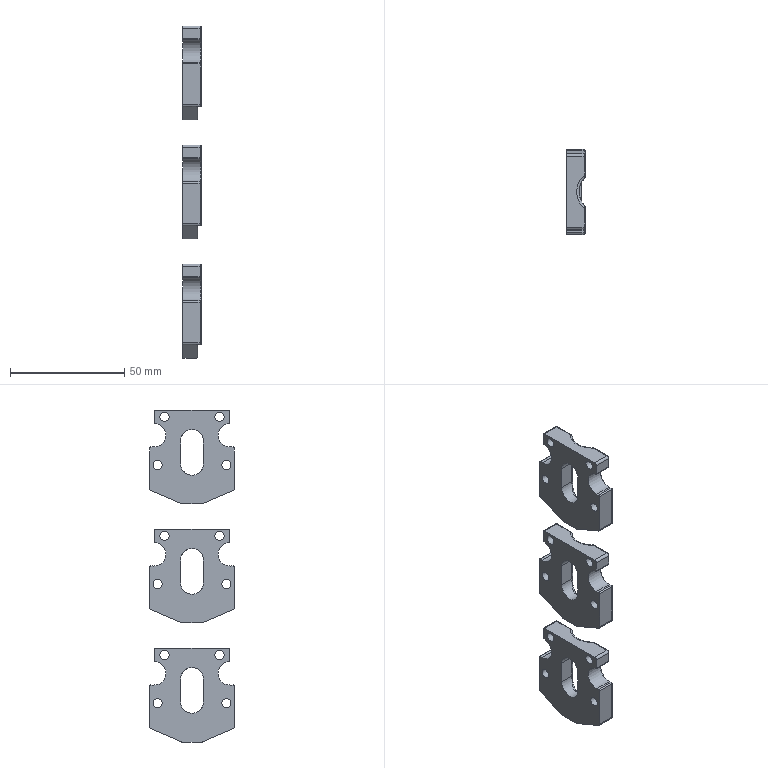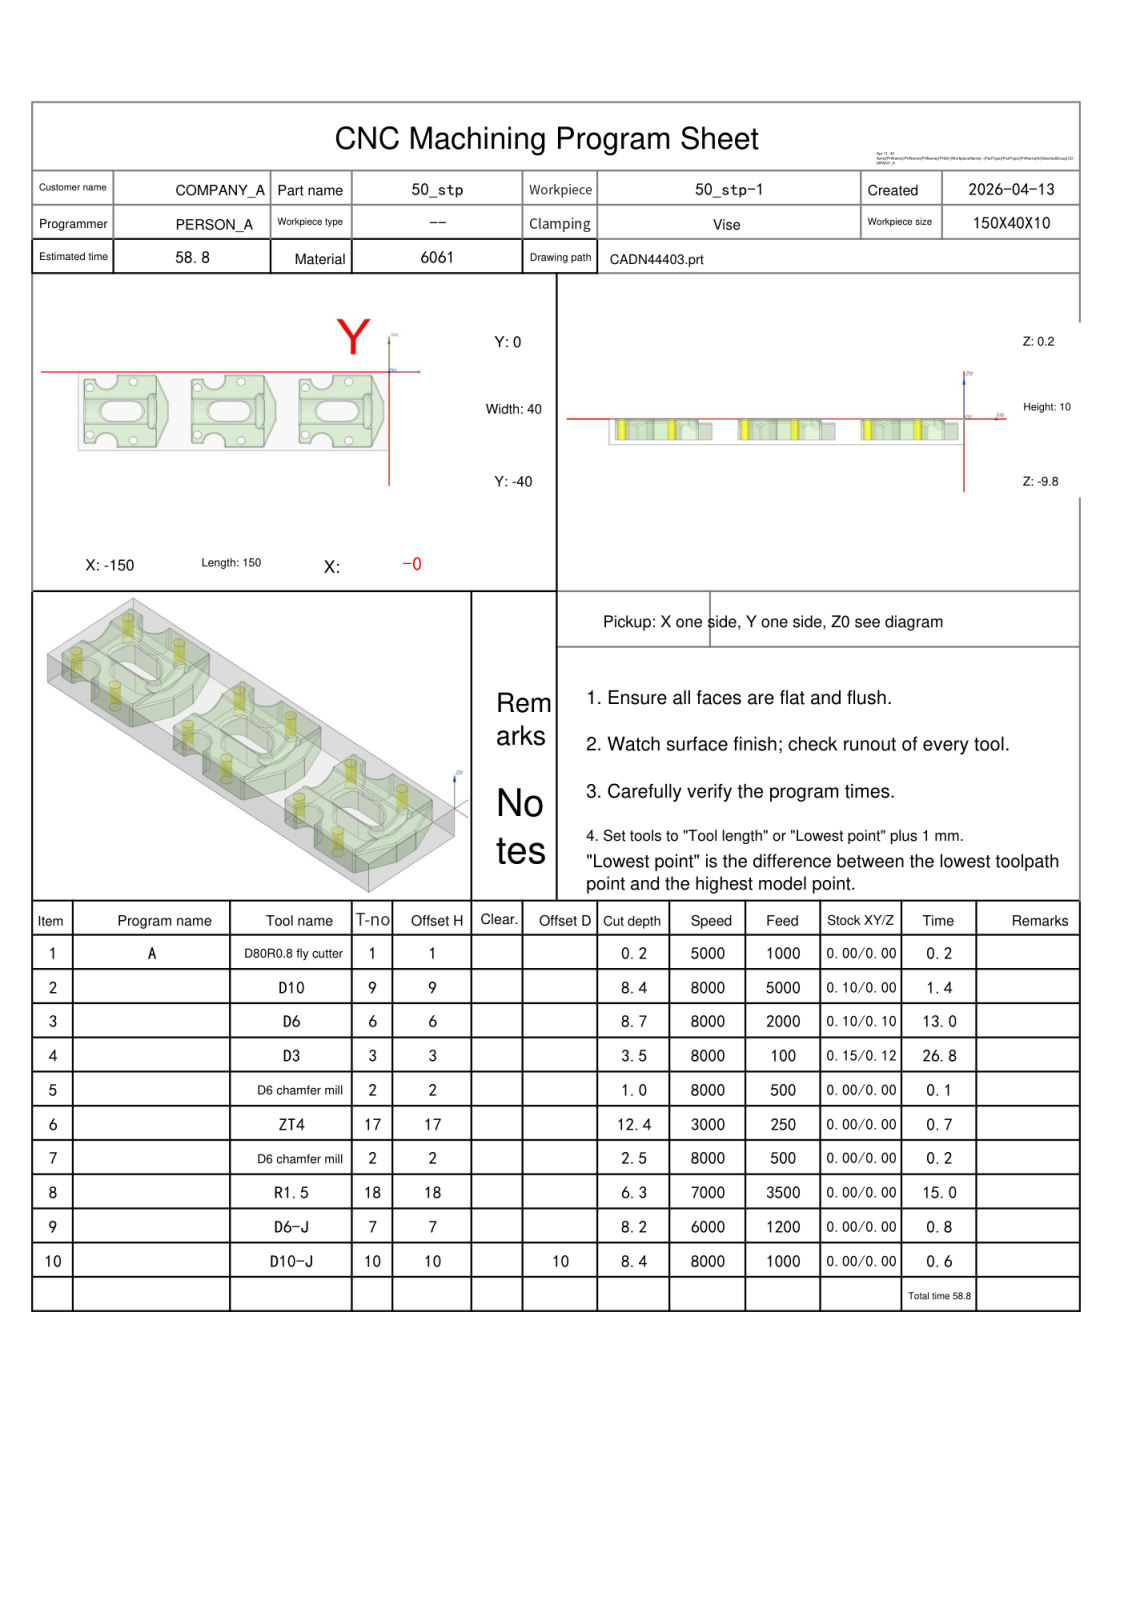NC program | NX | posted by the shop | part box 8 x 37 x 145 mm
Lines 1 to 1271 of 223411:
%
O0001
(Machine time: 60.56 MIN)
(===Total Tool:9===)
(T1=D80R0.8 fly cutter D=80.  R=0.8  D-  H01 Z=-0.   )
(T9=D10     D=10.  R=0.   D-  H09 Z=-8.2  )
(T6=D6      D=6.   R=0.   D-  H06 Z=-8.5  )
(T3=D3      D=3.   R=0.   D-  H03 Z=-3.31 )
(T2=D6 chamfer mill   D=6.   R=0.   D-  H02 Z=-2.3  )
(T17=ZT4    D=4.   DR_a=118 D-  H17 Z=-12.2 )
(T18=R1.5   D=3.   R=1.5  D-  H18 Z=-6.09 )
(T7=D6-J    D=6.   R=0.   D7  H07 Z=-8.   )
(T10=D10-J  D=10.  R=0.   D10 H10 Z=-8.2  )
G80 G90 G17 G49 G40
G91 G28 Z0
M01
N1 T01 M06
(D80R0.8 fly cutter  D=80. R=0.8 H=01 ce=0.00 di=0.00)
G00 G90 G54 X-192.5 Y-20. M03 S5000
G43 H01 Z20.
M08
Z2.
G01 Z0.0 F1000.
X-187.5
X37.5
X42.5
Z2.
G00 Z20.
G91 G28 Z0.0
M05
M09
G91 G28 Z0.0
M01
N2 T09 M06
(D10  D=10. R=0. H=09 ce=0.10 di=0.00)
G00 G90 G54 X-48.6 Y-20. M03 S8000
G43 H09 Z20.
M08
Z0.0
G01 Y-4.5 Z-.061 F5000.
G02 X-42.5 Y1.6 Z-.099 I6.1 J0.0
G01 X-38.128 Z-.117
G02 X-32.55 Y-3.504 Z-.149 I0.0 J-5.6
G01 X-32.549 Y-3.534
X-32.525 Y-3.554 Z-.15
X-32.496 Y-3.55
X-32.466
X-32.446 Y-3.527
X-32.45 Y-3.497
X-32.514 Y-2.3 Z-.155
G02 X-27.223 Y3.592 Z-.19 I5.592 J.3
X-26.922 Y3.6 Z-.191 I.3 J-5.592
G01 X-9.159 Z-.261
G02 X-3.553 Y-.097 Z-.289 I0.0 J-6.1
G01 X2.147 Y-13.397 Z-.346
G02 X2.6 Y-15.603 Z-.355 I-5.147 J-2.206
G01 Y-24.397 Z-.39
G02 X2.147 Y-26.603 Z-.399 I-5.6 J0.0
G01 X-3.553 Y-39.903 Z-.456
G02 X-9.159 Y-43.6 Z-.484 I-5.607 J2.403
G01 X-26.922 Z-.555
G02 X-32.522 Y-38. Z-.59 I0.0 J5.6
X-32.514 Y-37.7 Z-.591 I5.6 J0.0
G01 X-32.45 Y-36.503 Z-.595
X-32.447 Y-36.473 Z-.596
X-32.467 Y-36.45
X-32.497
X-32.527 Y-36.446
X-32.55 Y-36.466
Y-36.496
G02 X-38.128 Y-41.6 Z-.629 I-5.578 J.496
G01 X-42.5 Z-.646
G02 X-48.6 Y-35.5 Z-.684 I0.0 J6.1
G01 Y-4.5 Z-.807
G02 X-42.5 Y1.6 Z-.845 I6.1 J0.0
G01 X-38.128 Z-.862
G02 X-32.55 Y-3.504 Z-.895 I0.0 J-5.6
G01 X-32.549 Y-3.534
X-32.525 Y-3.554
X-32.496 Y-3.55
X-32.466
X-32.446 Y-3.527
X-32.45 Y-3.497
X-32.514 Y-2.3 Z-.9
G02 X-27.223 Y3.592 Z-.935 I5.592 J.3
X-26.922 Y3.6 Z-.936 I.3 J-5.592
G01 X-9.159 Z-1.006
G02 X-3.553 Y-.097 Z-1.035 I0.0 J-6.1
G01 X2.147 Y-13.397 Z-1.092
G02 X2.6 Y-15.603 Z-1.101 I-5.147 J-2.206
G01 Y-24.397 Z-1.136
G02 X2.147 Y-26.603 Z-1.145 I-5.6 J0.0
G01 X-3.553 Y-39.903 Z-1.202
G02 X-9.159 Y-43.6 Z-1.23 I-5.607 J2.403
G01 X-26.922 Z-1.3
G02 X-32.522 Y-38. Z-1.335 I0.0 J5.6
X-32.514 Y-37.7 Z-1.336 I5.6 J0.0
G01 X-32.45 Y-36.503 Z-1.341
X-32.447 Y-36.473
X-32.467 Y-36.45
X-32.497
X-32.527 Y-36.446
X-32.55 Y-36.466
Y-36.496 Z-1.342
G02 X-38.128 Y-41.6 Z-1.374 I-5.578 J.496
G01 X-42.5 Z-1.392
G02 X-48.6 Y-35.5 Z-1.43 I0.0 J6.1
G01 Y-4.5 Z-1.552
G02 X-42.5 Y1.6 Z-1.59 I6.1 J0.0
G01 X-38.128 Z-1.607
G02 X-32.55 Y-3.504 Z-1.64 I0.0 J-5.6
G01 X-32.549 Y-3.534
X-32.525 Y-3.554
X-32.496 Y-3.55 Z-1.641
X-32.466
X-32.446 Y-3.527
X-32.45 Y-3.497
X-32.514 Y-2.3 Z-1.646
G02 X-27.223 Y3.592 Z-1.68 I5.592 J.3
X-26.922 Y3.6 Z-1.682 I.3 J-5.592
G01 X-9.159 Z-1.752
G02 X-3.553 Y-.097 Z-1.78 I0.0 J-6.1
G01 X2.147 Y-13.397 Z-1.837
G02 X2.6 Y-15.603 Z-1.846 I-5.147 J-2.206
G01 Y-24.397 Z-1.881
G02 X2.147 Y-26.603 Z-1.89 I-5.6 J0.0
G01 X-3.553 Y-39.903 Z-1.947
G02 X-9.159 Y-43.6 Z-1.975 I-5.607 J2.403
G01 X-26.922 Z-2.046
G02 X-32.522 Y-38. Z-2.08 I0.0 J5.6
X-32.514 Y-37.7 Z-2.082 I5.6 J0.0
G01 X-32.45 Y-36.503 Z-2.086
X-32.447 Y-36.473
X-32.467 Y-36.45 Z-2.087
X-32.497
X-32.527 Y-36.446
X-32.55 Y-36.466
Y-36.496
G02 X-38.128 Y-41.6 Z-2.12 I-5.578 J.496
G01 X-42.5 Z-2.137
G02 X-48.6 Y-35.5 Z-2.175 I0.0 J6.1
G01 Y-4.5 Z-2.298
G02 X-42.5 Y1.6 Z-2.336 I6.1 J0.0
G01 X-38.128 Z-2.353
G02 X-32.55 Y-3.504 Z-2.386 I0.0 J-5.6
G01 X-32.549 Y-3.534
X-32.525 Y-3.554
X-32.496 Y-3.55
X-32.466
X-32.446 Y-3.527
X-32.45 Y-3.497
X-32.514 Y-2.3 Z-2.391
G02 X-27.223 Y3.592 Z-2.426 I5.592 J.3
X-26.922 Y3.6 Z-2.427 I.3 J-5.592
G01 X-9.159 Z-2.497
G02 X-3.553 Y-.097 Z-2.525 I0.0 J-6.1
G01 X2.147 Y-13.397 Z-2.583
G02 X2.6 Y-15.603 Z-2.592 I-5.147 J-2.206
G01 Y-24.397 Z-2.626
G02 X2.147 Y-26.603 Z-2.635 I-5.6 J0.0
G01 X-3.553 Y-39.903 Z-2.693
G02 X-9.159 Y-43.6 Z-2.721 I-5.607 J2.403
G01 X-26.922 Z-2.791
G02 X-32.522 Y-38. Z-2.826 I0.0 J5.6
X-32.514 Y-37.7 Z-2.827 I5.6 J0.0
G01 X-32.45 Y-36.503 Z-2.832
X-32.447 Y-36.473
X-32.467 Y-36.45
X-32.497
X-32.527 Y-36.446
X-32.55 Y-36.466
Y-36.496
G02 X-38.128 Y-41.6 Z-2.865 I-5.578 J.496
G01 X-42.5 Z-2.883
G02 X-48.6 Y-35.5 Z-2.92 I0.0 J6.1
G01 Y-4.5 Z-3.043
G02 X-42.5 Y1.6 Z-3.081 I6.1 J0.0
G01 X-38.128 Z-3.098
G02 X-32.55 Y-3.504 Z-3.131 I0.0 J-5.6
G01 X-32.549 Y-3.534
X-32.525 Y-3.554
X-32.496 Y-3.55
X-32.466 Z-3.132
X-32.446 Y-3.527
X-32.45 Y-3.497
X-32.514 Y-2.3 Z-3.137
G02 X-27.223 Y3.592 Z-3.171 I5.592 J.3
X-26.922 Y3.6 Z-3.173 I.3 J-5.592
G01 X-9.159 Z-3.243
G02 X-3.553 Y-.097 Z-3.271 I0.0 J-6.1
G01 X2.147 Y-13.397 Z-3.328
G02 X2.6 Y-15.603 Z-3.337 I-5.147 J-2.206
G01 Y-24.397 Z-3.372
G02 X2.147 Y-26.603 Z-3.381 I-5.6 J0.0
G01 X-3.553 Y-39.903 Z-3.438
G02 X-9.159 Y-43.6 Z-3.466 I-5.607 J2.403
G01 X-26.922 Z-3.537
G02 X-32.522 Y-38. Z-3.571 I0.0 J5.6
X-32.514 Y-37.7 Z-3.573 I5.6 J0.0
G01 X-32.45 Y-36.503 Z-3.577
X-32.447 Y-36.473
X-32.467 Y-36.45 Z-3.578
X-32.497
X-32.527 Y-36.446
X-32.55 Y-36.466
Y-36.496
G02 X-38.128 Y-41.6 Z-3.611 I-5.578 J.496
G01 X-42.5 Z-3.628
G02 X-48.6 Y-35.5 Z-3.666 I0.0 J6.1
G01 Y-4.5 Z-3.789
G02 X-42.5 Y1.6 Z-3.827 I6.1 J0.0
G01 X-38.128 Z-3.844
G02 X-32.55 Y-3.504 Z-3.877 I0.0 J-5.6
G01 X-32.549 Y-3.534
X-32.525 Y-3.554
X-32.496 Y-3.55
X-32.466
X-32.446 Y-3.527
X-32.45 Y-3.497
X-32.514 Y-2.3 Z-3.882
G02 X-27.223 Y3.592 Z-3.917 I5.592 J.3
X-26.922 Y3.6 Z-3.918 I.3 J-5.592
G01 X-9.159 Z-3.988
G02 X-3.553 Y-.097 Z-4.016 I0.0 J-6.1
G01 X2.147 Y-13.397 Z-4.074
G02 X2.6 Y-15.603 Z-4.083 I-5.147 J-2.206
G01 Y-24.397 Z-4.117
G02 X2.147 Y-26.603 Z-4.126 I-5.6 J0.0
G01 X-3.553 Y-39.903 Z-4.184
G02 X-9.159 Y-43.6 Z-4.212 I-5.607 J2.403
G01 X-26.922 Z-4.282
G02 X-32.522 Y-38. Z-4.317 I0.0 J5.6
X-32.514 Y-37.7 Z-4.318 I5.6 J0.0
G01 X-32.45 Y-36.503 Z-4.323
X-32.447 Y-36.473
X-32.467 Y-36.45
X-32.497
X-32.527 Y-36.446
X-32.55 Y-36.466
Y-36.496
G02 X-38.128 Y-41.6 Z-4.356 I-5.578 J.496
G01 X-42.5 Z-4.374
G02 X-48.6 Y-35.5 Z-4.411 I0.0 J6.1
G01 Y-4.5 Z-4.534
G02 X-42.5 Y1.6 Z-4.572 I6.1 J0.0
G01 X-38.128 Z-4.589
G02 X-32.55 Y-3.504 Z-4.622 I0.0 J-5.6
G01 X-32.549 Y-3.534
X-32.525 Y-3.554
X-32.496 Y-3.55
X-32.466 Z-4.623
X-32.446 Y-3.527
X-32.45 Y-3.497
X-32.514 Y-2.3 Z-4.627
G02 X-27.223 Y3.592 Z-4.662 I5.592 J.3
X-26.922 Y3.6 Z-4.663 I.3 J-5.592
G01 X-9.159 Z-4.734
G02 X-3.553 Y-.097 Z-4.762 I0.0 J-6.1
G01 X2.147 Y-13.397 Z-4.819
G02 X2.6 Y-15.603 Z-4.828 I-5.147 J-2.206
G01 Y-24.397 Z-4.863
G02 X2.147 Y-26.603 Z-4.872 I-5.6 J0.0
G01 X-3.553 Y-39.903 Z-4.929
G02 X-9.159 Y-43.6 Z-4.957 I-5.607 J2.403
G01 X-26.922 Z-5.027
G02 X-32.522 Y-38. Z-5.062 I0.0 J5.6
X-32.514 Y-37.7 Z-5.063 I5.6 J0.0
G01 X-32.45 Y-36.503 Z-5.068
X-32.447 Y-36.473
X-32.467 Y-36.45
X-32.497 Z-5.069
X-32.527 Y-36.446
X-32.55 Y-36.466
Y-36.496
G02 X-38.128 Y-41.6 Z-5.102 I-5.578 J.496
G01 X-42.5 Z-5.119
G02 X-48.6 Y-35.5 Z-5.157 I0.0 J6.1
G01 Y-4.5 Z-5.28
G02 X-42.5 Y1.6 Z-5.317 I6.1 J0.0
G01 X-38.128 Z-5.335
G02 X-32.55 Y-3.504 Z-5.368 I0.0 J-5.6
G01 X-32.549 Y-3.534
X-32.525 Y-3.554
X-32.496 Y-3.55
X-32.466
X-32.446 Y-3.527
X-32.45 Y-3.497
X-32.514 Y-2.3 Z-5.373
G02 X-27.223 Y3.592 Z-5.408 I5.592 J.3
X-26.922 Y3.6 Z-5.409 I.3 J-5.592
G01 X-9.159 Z-5.479
G02 X-3.553 Y-.097 Z-5.507 I0.0 J-6.1
G01 X2.147 Y-13.397 Z-5.565
G02 X2.6 Y-15.603 Z-5.574 I-5.147 J-2.206
G01 Y-24.397 Z-5.608
G02 X2.147 Y-26.603 Z-5.617 I-5.6 J0.0
G01 X-3.553 Y-39.903 Z-5.675
G02 X-9.159 Y-43.6 Z-5.703 I-5.607 J2.403
G01 X-26.922 Z-5.773
G02 X-32.522 Y-38. Z-5.808 I0.0 J5.6
X-32.514 Y-37.7 Z-5.809 I5.6 J0.0
G01 X-32.45 Y-36.503 Z-5.814
X-32.447 Y-36.473
X-32.467 Y-36.45
X-32.497
X-32.527 Y-36.446
X-32.55 Y-36.466
Y-36.496
G02 X-38.128 Y-41.6 Z-5.847 I-5.578 J.496
G01 X-42.5 Z-5.864
G02 X-48.6 Y-35.5 Z-5.902 I0.0 J6.1
G01 Y-4.5 Z-6.025
G02 X-42.5 Y1.6 Z-6.063 I6.1 J0.0
G01 X-38.128 Z-6.08
G02 X-32.55 Y-3.504 Z-6.113 I0.0 J-5.6
G01 X-32.549 Y-3.534
X-32.525 Y-3.554
X-32.496 Y-3.55
X-32.466
X-32.446 Y-3.527 Z-6.114
X-32.45 Y-3.497
X-32.514 Y-2.3 Z-6.118
G02 X-27.223 Y3.592 Z-6.153 I5.592 J.3
X-26.922 Y3.6 Z-6.154 I.3 J-5.592
G01 X-9.159 Z-6.225
G02 X-3.553 Y-.097 Z-6.253 I0.0 J-6.1
G01 X2.147 Y-13.397 Z-6.31
G02 X2.6 Y-15.603 Z-6.319 I-5.147 J-2.206
G01 Y-24.397 Z-6.354
G02 X2.147 Y-26.603 Z-6.363 I-5.6 J0.0
G01 X-3.553 Y-39.903 Z-6.42
G02 X-9.159 Y-43.6 Z-6.448 I-5.607 J2.403
G01 X-26.922 Z-6.518
G02 X-32.522 Y-38. Z-6.553 I0.0 J5.6
X-32.514 Y-37.7 Z-6.554 I5.6 J0.0
G01 X-32.45 Y-36.503 Z-6.559
X-32.447 Y-36.473
X-32.467 Y-36.45
X-32.497
X-32.527 Y-36.446 Z-6.56
X-32.55 Y-36.466
Y-36.496
G02 X-38.128 Y-41.6 Z-6.593 I-5.578 J.496
G01 X-42.5 Z-6.61
G02 X-48.6 Y-35.5 Z-6.648 I0.0 J6.1
G01 Y-4.5 Z-6.77
G02 X-42.5 Y1.6 Z-6.808 I6.1 J0.0
G01 X-38.128 Z-6.826
G02 X-32.55 Y-3.504 Z-6.858 I0.0 J-5.6
G01 X-32.549 Y-3.534 Z-6.859
X-32.525 Y-3.554
X-32.496 Y-3.55
X-32.466
X-32.446 Y-3.527
X-32.45 Y-3.497
X-32.514 Y-2.3 Z-6.864
G02 X-27.223 Y3.592 Z-6.899 I5.592 J.3
X-26.922 Y3.6 Z-6.9 I.3 J-5.592
G01 X-9.159 Z-6.97
G02 X-3.553 Y-.097 Z-6.998 I0.0 J-6.1
G01 X2.147 Y-13.397 Z-7.055
G02 X2.6 Y-15.603 Z-7.064 I-5.147 J-2.206
G01 Y-24.397 Z-7.099
G02 X2.147 Y-26.603 Z-7.108 I-5.6 J0.0
G01 X-3.553 Y-39.903 Z-7.165
G02 X-9.159 Y-43.6 Z-7.194 I-5.607 J2.403
G01 X-26.922 Z-7.264
G02 X-32.522 Y-38. Z-7.299 I0.0 J5.6
X-32.514 Y-37.7 Z-7.3 I5.6 J0.0
G01 X-32.45 Y-36.503 Z-7.305
X-32.447 Y-36.473
X-32.467 Y-36.45
X-32.497
X-32.527 Y-36.446
X-32.55 Y-36.466
Y-36.496
G02 X-38.128 Y-41.6 Z-7.338 I-5.578 J.496
G01 X-42.5 Z-7.355
G02 X-48.6 Y-35.5 Z-7.393 I0.0 J6.1
G01 Y-4.5 Z-7.516
G02 X-42.5 Y1.6 Z-7.554 I6.1 J0.0
G01 X-38.128 Z-7.571
G02 X-32.55 Y-3.504 Z-7.604 I0.0 J-5.6
G01 X-32.549 Y-3.534
X-32.525 Y-3.554
X-32.496 Y-3.55
X-32.466
X-32.446 Y-3.527
X-32.45 Y-3.497 Z-7.605
X-32.514 Y-2.3 Z-7.609
G02 X-27.223 Y3.592 Z-7.644 I5.592 J.3
X-26.922 Y3.6 Z-7.645 I.3 J-5.592
G01 X-9.159 Z-7.716
G02 X-3.553 Y-.097 Z-7.744 I0.0 J-6.1
G01 X2.147 Y-13.397 Z-7.801
G02 X2.6 Y-15.603 Z-7.81 I-5.147 J-2.206
G01 Y-24.397 Z-7.845
G02 X2.147 Y-26.603 Z-7.854 I-5.6 J0.0
G01 X-3.553 Y-39.903 Z-7.911
G02 X-9.159 Y-43.6 Z-7.939 I-5.607 J2.403
G01 X-26.922 Z-8.009
G02 X-32.522 Y-38. Z-8.044 I0.0 J5.6
X-32.514 Y-37.7 Z-8.045 I5.6 J0.0
G01 X-32.45 Y-36.503 Z-8.05
X-32.447 Y-36.473
X-32.467 Y-36.45
X-32.497
X-32.527 Y-36.446
X-32.55 Y-36.466 Z-8.051
Y-36.496
G02 X-38.128 Y-41.6 Z-8.083 I-5.578 J.496
G01 X-42.5 Z-8.101
G02 X-48.6 Y-35.5 Z-8.139 I0.0 J6.1
G01 Y-20. Z-8.2
Y-4.5
G02 X-42.5 Y1.6 I6.1 J0.0
G01 X-38.128
G02 X-32.55 Y-3.504 I0.0 J-5.6
G01 X-32.526 Y-3.554
X-32.467 Y-3.55
X-32.45 Y-3.497
X-32.514 Y-2.3
G02 X-32.522 Y-2. I5.592 J.3
X-26.922 Y3.6 I5.6 J0.0
G01 X-9.159
G02 X-3.553 Y-.097 I0.0 J-6.1
G01 X2.147 Y-13.397
G02 X2.6 Y-15.603 I-5.147 J-2.206
G01 Y-24.397
G02 X2.147 Y-26.603 I-5.6 J0.0
G01 X-3.553 Y-39.903
G02 X-9.159 Y-43.6 I-5.607 J2.403
G01 X-26.922
G02 X-32.522 Y-38. I0.0 J5.6
X-32.514 Y-37.7 I5.6 J0.0
G01 X-32.45 Y-36.503
X-32.467 Y-36.45
X-32.526 Y-36.446
X-32.55 Y-36.496
G02 X-38.128 Y-41.6 I-5.578 J.496
G01 X-42.5
G02 X-48.6 Y-35.5 I0.0 J6.1
G01 Y-20.
Y-19.5
Z-7.2
G00 Z20.
X-100.6 Y-20.
Z0.0
G01 Y-4.5 Z-.061
G02 X-94.5 Y1.6 Z-.099 I6.1 J0.0
G01 X-90.128 Z-.117
G02 X-84.55 Y-3.504 Z-.149 I0.0 J-5.6
G01 X-84.549 Y-3.534
X-84.525 Y-3.554 Z-.15
X-84.496 Y-3.55
X-84.466
X-84.446 Y-3.527
X-84.45 Y-3.497
X-84.514 Y-2.3 Z-.155
G02 X-79.223 Y3.592 Z-.19 I5.592 J.3
X-78.922 Y3.6 Z-.191 I.3 J-5.592
G01 X-61.159 Z-.261
G02 X-55.553 Y-.097 Z-.289 I0.0 J-6.1
G01 X-49.853 Y-13.397 Z-.346
G02 X-49.4 Y-15.603 Z-.355 I-5.147 J-2.206
G01 Y-24.397 Z-.39
G02 X-49.853 Y-26.603 Z-.399 I-5.6 J0.0
G01 X-55.553 Y-39.903 Z-.456
G02 X-61.159 Y-43.6 Z-.484 I-5.607 J2.403
G01 X-78.922 Z-.555
G02 X-84.522 Y-38. Z-.59 I0.0 J5.6
X-84.514 Y-37.7 Z-.591 I5.6 J0.0
G01 X-84.45 Y-36.503 Z-.595
X-84.447 Y-36.473 Z-.596
X-84.467 Y-36.45
X-84.497
X-84.527 Y-36.446
X-84.55 Y-36.466
Y-36.496
G02 X-90.128 Y-41.6 Z-.629 I-5.578 J.496
G01 X-94.5 Z-.646
G02 X-100.6 Y-35.5 Z-.684 I0.0 J6.1
G01 Y-4.5 Z-.807
G02 X-94.5 Y1.6 Z-.845 I6.1 J0.0
G01 X-90.128 Z-.862
G02 X-84.55 Y-3.504 Z-.895 I0.0 J-5.6
G01 X-84.549 Y-3.534
X-84.525 Y-3.554
X-84.496 Y-3.55
X-84.466
X-84.446 Y-3.527
X-84.45 Y-3.497
X-84.514 Y-2.3 Z-.9
G02 X-79.223 Y3.592 Z-.935 I5.592 J.3
X-78.922 Y3.6 Z-.936 I.3 J-5.592
G01 X-61.159 Z-1.006
G02 X-55.553 Y-.097 Z-1.035 I0.0 J-6.1
G01 X-49.853 Y-13.397 Z-1.092
G02 X-49.4 Y-15.603 Z-1.101 I-5.147 J-2.206
G01 Y-24.397 Z-1.136
G02 X-49.853 Y-26.603 Z-1.145 I-5.6 J0.0
G01 X-55.553 Y-39.903 Z-1.202
G02 X-61.159 Y-43.6 Z-1.23 I-5.607 J2.403
G01 X-78.922 Z-1.3
G02 X-84.522 Y-38. Z-1.335 I0.0 J5.6
X-84.514 Y-37.7 Z-1.336 I5.6 J0.0
G01 X-84.45 Y-36.503 Z-1.341
X-84.447 Y-36.473
X-84.467 Y-36.45
X-84.497
X-84.527 Y-36.446
X-84.55 Y-36.466
Y-36.496 Z-1.342
G02 X-90.128 Y-41.6 Z-1.374 I-5.578 J.496
G01 X-94.5 Z-1.392
G02 X-100.6 Y-35.5 Z-1.43 I0.0 J6.1
G01 Y-4.5 Z-1.552
G02 X-94.5 Y1.6 Z-1.59 I6.1 J0.0
G01 X-90.128 Z-1.607
G02 X-84.55 Y-3.504 Z-1.64 I0.0 J-5.6
G01 X-84.549 Y-3.534
X-84.525 Y-3.554
X-84.496 Y-3.55 Z-1.641
X-84.466
X-84.446 Y-3.527
X-84.45 Y-3.497
X-84.514 Y-2.3 Z-1.646
G02 X-79.223 Y3.592 Z-1.68 I5.592 J.3
X-78.922 Y3.6 Z-1.682 I.3 J-5.592
G01 X-61.159 Z-1.752
G02 X-55.553 Y-.097 Z-1.78 I0.0 J-6.1
G01 X-49.853 Y-13.397 Z-1.837
G02 X-49.4 Y-15.603 Z-1.846 I-5.147 J-2.206
G01 Y-24.397 Z-1.881
G02 X-49.853 Y-26.603 Z-1.89 I-5.6 J0.0
G01 X-55.553 Y-39.903 Z-1.947
G02 X-61.159 Y-43.6 Z-1.975 I-5.607 J2.403
G01 X-78.922 Z-2.046
G02 X-84.522 Y-38. Z-2.08 I0.0 J5.6
X-84.514 Y-37.7 Z-2.082 I5.6 J0.0
G01 X-84.45 Y-36.503 Z-2.086
X-84.447 Y-36.473
X-84.467 Y-36.45 Z-2.087
X-84.497
X-84.527 Y-36.446
X-84.55 Y-36.466
Y-36.496
G02 X-90.128 Y-41.6 Z-2.12 I-5.578 J.496
G01 X-94.5 Z-2.137
G02 X-100.6 Y-35.5 Z-2.175 I0.0 J6.1
G01 Y-4.5 Z-2.298
G02 X-94.5 Y1.6 Z-2.336 I6.1 J0.0
G01 X-90.128 Z-2.353
G02 X-84.55 Y-3.504 Z-2.386 I0.0 J-5.6
G01 X-84.549 Y-3.534
X-84.525 Y-3.554
X-84.496 Y-3.55
X-84.466
X-84.446 Y-3.527
X-84.45 Y-3.497
X-84.514 Y-2.3 Z-2.391
G02 X-79.223 Y3.592 Z-2.426 I5.592 J.3
X-78.922 Y3.6 Z-2.427 I.3 J-5.592
G01 X-61.159 Z-2.497
G02 X-55.553 Y-.097 Z-2.525 I0.0 J-6.1
G01 X-49.853 Y-13.397 Z-2.583
G02 X-49.4 Y-15.603 Z-2.592 I-5.147 J-2.206
G01 Y-24.397 Z-2.626
G02 X-49.853 Y-26.603 Z-2.635 I-5.6 J0.0
G01 X-55.553 Y-39.903 Z-2.693
G02 X-61.159 Y-43.6 Z-2.721 I-5.607 J2.403
G01 X-78.922 Z-2.791
G02 X-84.522 Y-38. Z-2.826 I0.0 J5.6
X-84.514 Y-37.7 Z-2.827 I5.6 J0.0
G01 X-84.45 Y-36.503 Z-2.832
X-84.447 Y-36.473
X-84.467 Y-36.45
X-84.497
X-84.527 Y-36.446
X-84.55 Y-36.466
Y-36.496
G02 X-90.128 Y-41.6 Z-2.865 I-5.578 J.496
G01 X-94.5 Z-2.883
G02 X-100.6 Y-35.5 Z-2.92 I0.0 J6.1
G01 Y-4.5 Z-3.043
G02 X-94.5 Y1.6 Z-3.081 I6.1 J0.0
G01 X-90.128 Z-3.098
G02 X-84.55 Y-3.504 Z-3.131 I0.0 J-5.6
G01 X-84.549 Y-3.534
X-84.525 Y-3.554
X-84.496 Y-3.55
X-84.466 Z-3.132
X-84.446 Y-3.527
X-84.45 Y-3.497
X-84.514 Y-2.3 Z-3.137
G02 X-79.223 Y3.592 Z-3.171 I5.592 J.3
X-78.922 Y3.6 Z-3.173 I.3 J-5.592
G01 X-61.159 Z-3.243
G02 X-55.553 Y-.097 Z-3.271 I0.0 J-6.1
G01 X-49.853 Y-13.397 Z-3.328
G02 X-49.4 Y-15.603 Z-3.337 I-5.147 J-2.206
G01 Y-24.397 Z-3.372
G02 X-49.853 Y-26.603 Z-3.381 I-5.6 J0.0
G01 X-55.553 Y-39.903 Z-3.438
G02 X-61.159 Y-43.6 Z-3.466 I-5.607 J2.403
G01 X-78.922 Z-3.537
G02 X-84.522 Y-38. Z-3.571 I0.0 J5.6
X-84.514 Y-37.7 Z-3.573 I5.6 J0.0
G01 X-84.45 Y-36.503 Z-3.577
X-84.447 Y-36.473
X-84.467 Y-36.45 Z-3.578
X-84.497
X-84.527 Y-36.446
X-84.55 Y-36.466
Y-36.496
G02 X-90.128 Y-41.6 Z-3.611 I-5.578 J.496
G01 X-94.5 Z-3.628
G02 X-100.6 Y-35.5 Z-3.666 I0.0 J6.1
G01 Y-4.5 Z-3.789
G02 X-94.5 Y1.6 Z-3.827 I6.1 J0.0
G01 X-90.128 Z-3.844
G02 X-84.55 Y-3.504 Z-3.877 I0.0 J-5.6
G01 X-84.549 Y-3.534
X-84.525 Y-3.554
X-84.496 Y-3.55
X-84.466
X-84.446 Y-3.527
X-84.45 Y-3.497
X-84.514 Y-2.3 Z-3.882
G02 X-79.223 Y3.592 Z-3.917 I5.592 J.3
X-78.922 Y3.6 Z-3.918 I.3 J-5.592
G01 X-61.159 Z-3.988
G02 X-55.553 Y-.097 Z-4.016 I0.0 J-6.1
G01 X-49.853 Y-13.397 Z-4.074
G02 X-49.4 Y-15.603 Z-4.083 I-5.147 J-2.206
G01 Y-24.397 Z-4.117
G02 X-49.853 Y-26.603 Z-4.126 I-5.6 J0.0
G01 X-55.553 Y-39.903 Z-4.184
G02 X-61.159 Y-43.6 Z-4.212 I-5.607 J2.403
G01 X-78.922 Z-4.282
G02 X-84.522 Y-38. Z-4.317 I0.0 J5.6
X-84.514 Y-37.7 Z-4.318 I5.6 J0.0
G01 X-84.45 Y-36.503 Z-4.323
X-84.447 Y-36.473
X-84.467 Y-36.45
X-84.497
X-84.527 Y-36.446
X-84.55 Y-36.466
Y-36.496
G02 X-90.128 Y-41.6 Z-4.356 I-5.578 J.496
G01 X-94.5 Z-4.374
G02 X-100.6 Y-35.5 Z-4.411 I0.0 J6.1
G01 Y-4.5 Z-4.534
G02 X-94.5 Y1.6 Z-4.572 I6.1 J0.0
G01 X-90.128 Z-4.589
G02 X-84.55 Y-3.504 Z-4.622 I0.0 J-5.6
G01 X-84.549 Y-3.534
X-84.525 Y-3.554
X-84.496 Y-3.55
X-84.466 Z-4.623
X-84.446 Y-3.527
X-84.45 Y-3.497
X-84.514 Y-2.3 Z-4.627
G02 X-79.223 Y3.592 Z-4.662 I5.592 J.3
X-78.922 Y3.6 Z-4.663 I.3 J-5.592
G01 X-61.159 Z-4.734
G02 X-55.553 Y-.097 Z-4.762 I0.0 J-6.1
G01 X-49.853 Y-13.397 Z-4.819
G02 X-49.4 Y-15.603 Z-4.828 I-5.147 J-2.206
G01 Y-24.397 Z-4.863
G02 X-49.853 Y-26.603 Z-4.872 I-5.6 J0.0
G01 X-55.553 Y-39.903 Z-4.929
G02 X-61.159 Y-43.6 Z-4.957 I-5.607 J2.403
G01 X-78.922 Z-5.027
G02 X-84.522 Y-38. Z-5.062 I0.0 J5.6
X-84.514 Y-37.7 Z-5.063 I5.6 J0.0
G01 X-84.45 Y-36.503 Z-5.068
X-84.447 Y-36.473
X-84.467 Y-36.45
X-84.497 Z-5.069
X-84.527 Y-36.446
X-84.55 Y-36.466
Y-36.496
G02 X-90.128 Y-41.6 Z-5.102 I-5.578 J.496
G01 X-94.5 Z-5.119
G02 X-100.6 Y-35.5 Z-5.157 I0.0 J6.1
G01 Y-4.5 Z-5.28
G02 X-94.5 Y1.6 Z-5.317 I6.1 J0.0
G01 X-90.128 Z-5.335
G02 X-84.55 Y-3.504 Z-5.368 I0.0 J-5.6
G01 X-84.549 Y-3.534
X-84.525 Y-3.554
X-84.496 Y-3.55
X-84.466
X-84.446 Y-3.527
X-84.45 Y-3.497
X-84.514 Y-2.3 Z-5.373
G02 X-79.223 Y3.592 Z-5.408 I5.592 J.3
X-78.922 Y3.6 Z-5.409 I.3 J-5.592
G01 X-61.159 Z-5.479
G02 X-55.553 Y-.097 Z-5.507 I0.0 J-6.1
G01 X-49.853 Y-13.397 Z-5.565
G02 X-49.4 Y-15.603 Z-5.574 I-5.147 J-2.206
G01 Y-24.397 Z-5.608
G02 X-49.853 Y-26.603 Z-5.617 I-5.6 J0.0
G01 X-55.553 Y-39.903 Z-5.675
G02 X-61.159 Y-43.6 Z-5.703 I-5.607 J2.403
G01 X-78.922 Z-5.773
G02 X-84.522 Y-38. Z-5.808 I0.0 J5.6
X-84.514 Y-37.7 Z-5.809 I5.6 J0.0
G01 X-84.45 Y-36.503 Z-5.814
X-84.447 Y-36.473
X-84.467 Y-36.45
X-84.497
X-84.527 Y-36.446
X-84.55 Y-36.466
Y-36.496
G02 X-90.128 Y-41.6 Z-5.847 I-5.578 J.496
G01 X-94.5 Z-5.864
G02 X-100.6 Y-35.5 Z-5.902 I0.0 J6.1
G01 Y-4.5 Z-6.025
G02 X-94.5 Y1.6 Z-6.063 I6.1 J0.0
G01 X-90.128 Z-6.08
G02 X-84.55 Y-3.504 Z-6.113 I0.0 J-5.6
G01 X-84.549 Y-3.534
X-84.525 Y-3.554
X-84.496 Y-3.55
X-84.466
X-84.446 Y-3.527 Z-6.114
X-84.45 Y-3.497
X-84.514 Y-2.3 Z-6.118
G02 X-79.223 Y3.592 Z-6.153 I5.592 J.3
X-78.922 Y3.6 Z-6.154 I.3 J-5.592
G01 X-61.159 Z-6.225
G02 X-55.553 Y-.097 Z-6.253 I0.0 J-6.1
G01 X-49.853 Y-13.397 Z-6.31
G02 X-49.4 Y-15.603 Z-6.319 I-5.147 J-2.206
G01 Y-24.397 Z-6.354
G02 X-49.853 Y-26.603 Z-6.363 I-5.6 J0.0
G01 X-55.553 Y-39.903 Z-6.42
G02 X-61.159 Y-43.6 Z-6.448 I-5.607 J2.403
G01 X-78.922 Z-6.518
G02 X-84.522 Y-38. Z-6.553 I0.0 J5.6
X-84.514 Y-37.7 Z-6.554 I5.6 J0.0
G01 X-84.45 Y-36.503 Z-6.559
X-84.447 Y-36.473
X-84.467 Y-36.45
X-84.497
X-84.527 Y-36.446 Z-6.56
X-84.55 Y-36.466
Y-36.496
G02 X-90.128 Y-41.6 Z-6.593 I-5.578 J.496
G01 X-94.5 Z-6.61
G02 X-100.6 Y-35.5 Z-6.648 I0.0 J6.1
G01 Y-4.5 Z-6.77
G02 X-94.5 Y1.6 Z-6.808 I6.1 J0.0
G01 X-90.128 Z-6.826
G02 X-84.55 Y-3.504 Z-6.858 I0.0 J-5.6
G01 X-84.549 Y-3.534 Z-6.859
X-84.525 Y-3.554
X-84.496 Y-3.55
X-84.466
X-84.446 Y-3.527
X-84.45 Y-3.497
X-84.514 Y-2.3 Z-6.864
G02 X-79.223 Y3.592 Z-6.899 I5.592 J.3
X-78.922 Y3.6 Z-6.9 I.3 J-5.592
G01 X-61.159 Z-6.97
G02 X-55.553 Y-.097 Z-6.998 I0.0 J-6.1
G01 X-49.853 Y-13.397 Z-7.055
G02 X-49.4 Y-15.603 Z-7.064 I-5.147 J-2.206
G01 Y-24.397 Z-7.099
G02 X-49.853 Y-26.603 Z-7.108 I-5.6 J0.0
G01 X-55.553 Y-39.903 Z-7.165
G02 X-61.159 Y-43.6 Z-7.194 I-5.607 J2.403
G01 X-78.922 Z-7.264
G02 X-84.522 Y-38. Z-7.299 I0.0 J5.6
X-84.514 Y-37.7 Z-7.3 I5.6 J0.0
G01 X-84.45 Y-36.503 Z-7.305
X-84.447 Y-36.473
X-84.467 Y-36.45
X-84.497
X-84.527 Y-36.446
X-84.55 Y-36.466
Y-36.496
G02 X-90.128 Y-41.6 Z-7.338 I-5.578 J.496
G01 X-94.5 Z-7.355
G02 X-100.6 Y-35.5 Z-7.393 I0.0 J6.1
G01 Y-4.5 Z-7.516
G02 X-94.5 Y1.6 Z-7.554 I6.1 J0.0
G01 X-90.128 Z-7.571
G02 X-84.55 Y-3.504 Z-7.604 I0.0 J-5.6
G01 X-84.549 Y-3.534
X-84.525 Y-3.554
X-84.496 Y-3.55
X-84.466
X-84.446 Y-3.527
X-84.45 Y-3.497 Z-7.605
X-84.514 Y-2.3 Z-7.609
G02 X-79.223 Y3.592 Z-7.644 I5.592 J.3
X-78.922 Y3.6 Z-7.645 I.3 J-5.592
G01 X-61.159 Z-7.716
G02 X-55.553 Y-.097 Z-7.744 I0.0 J-6.1
G01 X-49.853 Y-13.397 Z-7.801
G02 X-49.4 Y-15.603 Z-7.81 I-5.147 J-2.206
G01 Y-24.397 Z-7.845
G02 X-49.853 Y-26.603 Z-7.854 I-5.6 J0.0
G01 X-55.553 Y-39.903 Z-7.911
G02 X-61.159 Y-43.6 Z-7.939 I-5.607 J2.403
G01 X-78.922 Z-8.009
G02 X-84.522 Y-38. Z-8.044 I0.0 J5.6
X-84.514 Y-37.7 Z-8.045 I5.6 J0.0
G01 X-84.45 Y-36.503 Z-8.05
X-84.447 Y-36.473
X-84.467 Y-36.45
X-84.497
X-84.527 Y-36.446
X-84.55 Y-36.466 Z-8.051
Y-36.496
G02 X-90.128 Y-41.6 Z-8.083 I-5.578 J.496
G01 X-94.5 Z-8.101
G02 X-100.6 Y-35.5 Z-8.139 I0.0 J6.1
G01 Y-20. Z-8.2
Y-4.5
G02 X-94.5 Y1.6 I6.1 J0.0
G01 X-90.128
G02 X-84.55 Y-3.504 I0.0 J-5.6
G01 X-84.526 Y-3.554
X-84.467 Y-3.55
X-84.45 Y-3.497
X-84.514 Y-2.3
G02 X-84.522 Y-2. I5.592 J.3
X-78.922 Y3.6 I5.6 J0.0
G01 X-61.159
G02 X-55.553 Y-.097 I0.0 J-6.1
G01 X-49.853 Y-13.397
G02 X-49.4 Y-15.603 I-5.147 J-2.206
G01 Y-24.397
G02 X-49.853 Y-26.603 I-5.6 J0.0
G01 X-55.553 Y-39.903
G02 X-61.159 Y-43.6 I-5.607 J2.403
G01 X-78.922
G02 X-84.522 Y-38. I0.0 J5.6
X-84.514 Y-37.7 I5.6 J0.0
G01 X-84.45 Y-36.503
X-84.467 Y-36.45
X-84.526 Y-36.446
X-84.55 Y-36.496
G02 X-90.128 Y-41.6 I-5.578 J.496
G01 X-94.5
G02 X-100.6 Y-35.5 I0.0 J6.1
G01 Y-20.
Y-19.5
Z-7.2
G00 Z20.
X-152.6 Y-20.
Z0.0
G01 Y-4.5 Z-.061
G02 X-146.5 Y1.6 Z-.099 I6.1 J0.0
G01 X-142.128 Z-.117
G02 X-136.55 Y-3.504 Z-.149 I0.0 J-5.6
G01 X-136.549 Y-3.534
X-136.525 Y-3.554 Z-.15
X-136.496 Y-3.55
X-136.466
X-136.446 Y-3.527
X-136.45 Y-3.497
X-136.514 Y-2.3 Z-.155
G02 X-131.223 Y3.592 Z-.19 I5.592 J.3
X-130.922 Y3.6 Z-.191 I.3 J-5.592
G01 X-113.159 Z-.261
G02 X-107.553 Y-.097 Z-.289 I0.0 J-6.1
G01 X-101.853 Y-13.397 Z-.346
G02 X-101.4 Y-15.603 Z-.355 I-5.147 J-2.206
G01 Y-24.397 Z-.39
G02 X-101.853 Y-26.603 Z-.399 I-5.6 J0.0
G01 X-107.553 Y-39.903 Z-.456
G02 X-113.159 Y-43.6 Z-.484 I-5.607 J2.403
G01 X-130.922 Z-.555
G02 X-136.522 Y-38. Z-.59 I0.0 J5.6
X-136.514 Y-37.7 Z-.591 I5.6 J0.0
G01 X-136.45 Y-36.503 Z-.595
X-136.447 Y-36.473 Z-.596
X-136.467 Y-36.45
X-136.497
X-136.527 Y-36.446
X-136.55 Y-36.466
Y-36.496
G02 X-142.128 Y-41.6 Z-.629 I-5.578 J.496
G01 X-146.5 Z-.646
G02 X-152.6 Y-35.5 Z-.684 I0.0 J6.1
G01 Y-4.5 Z-.807
G02 X-146.5 Y1.6 Z-.845 I6.1 J0.0
G01 X-142.128 Z-.862
G02 X-136.55 Y-3.504 Z-.895 I0.0 J-5.6
G01 X-136.549 Y-3.534
X-136.525 Y-3.554
X-136.496 Y-3.55
X-136.466
X-136.446 Y-3.527
X-136.45 Y-3.497
X-136.514 Y-2.3 Z-.9
G02 X-131.223 Y3.592 Z-.935 I5.592 J.3
X-130.922 Y3.6 Z-.936 I.3 J-5.592
G01 X-113.159 Z-1.006
G02 X-107.553 Y-.097 Z-1.035 I0.0 J-6.1
G01 X-101.853 Y-13.397 Z-1.092
G02 X-101.4 Y-15.603 Z-1.101 I-5.147 J-2.206
G01 Y-24.397 Z-1.136
G02 X-101.853 Y-26.603 Z-1.145 I-5.6 J0.0
G01 X-107.553 Y-39.903 Z-1.202
G02 X-113.159 Y-43.6 Z-1.23 I-5.607 J2.403
G01 X-130.922 Z-1.3
G02 X-136.522 Y-38. Z-1.335 I0.0 J5.6
X-136.514 Y-37.7 Z-1.336 I5.6 J0.0
G01 X-136.45 Y-36.503 Z-1.341
X-136.447 Y-36.473
X-136.467 Y-36.45
X-136.497
X-136.527 Y-36.446
X-136.55 Y-36.466
Y-36.496 Z-1.342
G02 X-142.128 Y-41.6 Z-1.374 I-5.578 J.496
G01 X-146.5 Z-1.392
G02 X-152.6 Y-35.5 Z-1.43 I0.0 J6.1
G01 Y-4.5 Z-1.552
G02 X-146.5 Y1.6 Z-1.59 I6.1 J0.0
G01 X-142.128 Z-1.607
G02 X-136.55 Y-3.504 Z-1.64 I0.0 J-5.6
G01 X-136.549 Y-3.534
X-136.525 Y-3.554
X-136.496 Y-3.55 Z-1.641
X-136.466
X-136.446 Y-3.527
X-136.45 Y-3.497
X-136.514 Y-2.3 Z-1.646
G02 X-131.223 Y3.592 Z-1.68 I5.592 J.3
X-130.922 Y3.6 Z-1.682 I.3 J-5.592
G01 X-113.159 Z-1.752
G02 X-107.553 Y-.097 Z-1.78 I0.0 J-6.1
G01 X-101.853 Y-13.397 Z-1.837
G02 X-101.4 Y-15.603 Z-1.846 I-5.147 J-2.206
G01 Y-24.397 Z-1.881
G02 X-101.853 Y-26.603 Z-1.89 I-5.6 J0.0
G01 X-107.553 Y-39.903 Z-1.947
G02 X-113.159 Y-43.6 Z-1.975 I-5.607 J2.403
G01 X-130.922 Z-2.046
G02 X-136.522 Y-38. Z-2.08 I0.0 J5.6
X-136.514 Y-37.7 Z-2.082 I5.6 J0.0
G01 X-136.45 Y-36.503 Z-2.086
X-136.447 Y-36.473
X-136.467 Y-36.45 Z-2.087
X-136.497
X-136.527 Y-36.446
X-136.55 Y-36.466
Y-36.496
G02 X-142.128 Y-41.6 Z-2.12 I-5.578 J.496
G01 X-146.5 Z-2.137
G02 X-152.6 Y-35.5 Z-2.175 I0.0 J6.1
G01 Y-4.5 Z-2.298
G02 X-146.5 Y1.6 Z-2.336 I6.1 J0.0
G01 X-142.128 Z-2.353
G02 X-136.55 Y-3.504 Z-2.386 I0.0 J-5.6
G01 X-136.549 Y-3.534
X-136.525 Y-3.554
X-136.496 Y-3.55
X-136.466
X-136.446 Y-3.527
X-136.45 Y-3.497
X-136.514 Y-2.3 Z-2.391
G02 X-131.223 Y3.592 Z-2.426 I5.592 J.3
X-130.922 Y3.6 Z-2.427 I.3 J-5.592
G01 X-113.159 Z-2.497
G02 X-107.553 Y-.097 Z-2.525 I0.0 J-6.1
G01 X-101.853 Y-13.397 Z-2.583
G02 X-101.4 Y-15.603 Z-2.592 I-5.147 J-2.206
G01 Y-24.397 Z-2.626
G02 X-101.853 Y-26.603 Z-2.635 I-5.6 J0.0
G01 X-107.553 Y-39.903 Z-2.693
G02 X-113.159 Y-43.6 Z-2.721 I-5.607 J2.403
G01 X-130.922 Z-2.791
G02 X-136.522 Y-38. Z-2.826 I0.0 J5.6
X-136.514 Y-37.7 Z-2.827 I5.6 J0.0
G01 X-136.45 Y-36.503 Z-2.832
X-136.447 Y-36.473
X-136.467 Y-36.45
X-136.497
X-136.527 Y-36.446
X-136.55 Y-36.466
Y-36.496
G02 X-142.128 Y-41.6 Z-2.865 I-5.578 J.496
G01 X-146.5 Z-2.883
G02 X-152.6 Y-35.5 Z-2.92 I0.0 J6.1
G01 Y-4.5 Z-3.043
G02 X-146.5 Y1.6 Z-3.081 I6.1 J0.0
G01 X-142.128 Z-3.098
G02 X-136.55 Y-3.504 Z-3.131 I0.0 J-5.6
G01 X-136.549 Y-3.534
X-136.525 Y-3.554
X-136.496 Y-3.55
X-136.466 Z-3.132
X-136.446 Y-3.527
X-136.45 Y-3.497
X-136.514 Y-2.3 Z-3.137
G02 X-131.223 Y3.592 Z-3.171 I5.592 J.3
X-130.922 Y3.6 Z-3.173 I.3 J-5.592
G01 X-113.159 Z-3.243
G02 X-107.553 Y-.097 Z-3.271 I0.0 J-6.1
G01 X-101.853 Y-13.397 Z-3.328
G02 X-101.4 Y-15.603 Z-3.337 I-5.147 J-2.206
G01 Y-24.397 Z-3.372
G02 X-101.853 Y-26.603 Z-3.381 I-5.6 J0.0
G01 X-107.553 Y-39.903 Z-3.438
G02 X-113.159 Y-43.6 Z-3.466 I-5.607 J2.403
G01 X-130.922 Z-3.537
G02 X-136.522 Y-38. Z-3.571 I0.0 J5.6
X-136.514 Y-37.7 Z-3.573 I5.6 J0.0
G01 X-136.45 Y-36.503 Z-3.577
X-136.447 Y-36.473
X-136.467 Y-36.45 Z-3.578
X-136.497
X-136.527 Y-36.446
X-136.55 Y-36.466
Y-36.496
G02 X-142.128 Y-41.6 Z-3.611 I-5.578 J.496
G01 X-146.5 Z-3.628
G02 X-152.6 Y-35.5 Z-3.666 I0.0 J6.1
G01 Y-4.5 Z-3.789
G02 X-146.5 Y1.6 Z-3.827 I6.1 J0.0
G01 X-142.128 Z-3.844
G02 X-136.55 Y-3.504 Z-3.877 I0.0 J-5.6
G01 X-136.549 Y-3.534
X-136.525 Y-3.554
X-136.496 Y-3.55
X-136.466
X-136.446 Y-3.527
X-136.45 Y-3.497
X-136.514 Y-2.3 Z-3.882
G02 X-131.223 Y3.592 Z-3.917 I5.592 J.3
X-130.922 Y3.6 Z-3.918 I.3 J-5.592
G01 X-113.159 Z-3.988
G02 X-107.553 Y-.097 Z-4.016 I0.0 J-6.1
G01 X-101.853 Y-13.397 Z-4.074
G02 X-101.4 Y-15.603 Z-4.083 I-5.147 J-2.206
G01 Y-24.397 Z-4.117
G02 X-101.853 Y-26.603 Z-4.126 I-5.6 J0.0
G01 X-107.553 Y-39.903 Z-4.184
G02 X-113.159 Y-43.6 Z-4.212 I-5.607 J2.403
G01 X-130.922 Z-4.282
G02 X-136.522 Y-38. Z-4.317 I0.0 J5.6
X-136.514 Y-37.7 Z-4.318 I5.6 J0.0
G01 X-136.45 Y-36.503 Z-4.323
X-136.447 Y-36.473
X-136.467 Y-36.45
X-136.497
X-136.527 Y-36.446
X-136.55 Y-36.466
Y-36.496
G02 X-142.128 Y-41.6 Z-4.356 I-5.578 J.496
G01 X-146.5 Z-4.374
G02 X-152.6 Y-35.5 Z-4.411 I0.0 J6.1
G01 Y-4.5 Z-4.534
G02 X-146.5 Y1.6 Z-4.572 I6.1 J0.0
G01 X-142.128 Z-4.589
G02 X-136.55 Y-3.504 Z-4.622 I0.0 J-5.6
G01 X-136.549 Y-3.534
X-136.525 Y-3.554
X-136.496 Y-3.55
X-136.466 Z-4.623
X-136.446 Y-3.527
X-136.45 Y-3.497
X-136.514 Y-2.3 Z-4.627
G02 X-131.223 Y3.592 Z-4.662 I5.592 J.3
X-130.922 Y3.6 Z-4.663 I.3 J-5.592
G01 X-113.159 Z-4.734
G02 X-107.553 Y-.097 Z-4.762 I0.0 J-6.1
G01 X-101.853 Y-13.397 Z-4.819
G02 X-101.4 Y-15.603 Z-4.828 I-5.147 J-2.206
G01 Y-24.397 Z-4.863
G02 X-101.853 Y-26.603 Z-4.872 I-5.6 J0.0
G01 X-107.553 Y-39.903 Z-4.929
G02 X-113.159 Y-43.6 Z-4.957 I-5.607 J2.403
G01 X-130.922 Z-5.027
G02 X-136.522 Y-38. Z-5.062 I0.0 J5.6
X-136.514 Y-37.7 Z-5.063 I5.6 J0.0
G01 X-136.45 Y-36.503 Z-5.068
X-136.447 Y-36.473
X-136.467 Y-36.45
X-136.497 Z-5.069
X-136.527 Y-36.446
X-136.55 Y-36.466
Y-36.496
G02 X-142.128 Y-41.6 Z-5.102 I-5.578 J.496
G01 X-146.5 Z-5.119
G02 X-152.6 Y-35.5 Z-5.157 I0.0 J6.1
G01 Y-4.5 Z-5.28
G02 X-146.5 Y1.6 Z-5.317 I6.1 J0.0
G01 X-142.128 Z-5.335
G02 X-136.55 Y-3.504 Z-5.368 I0.0 J-5.6
G01 X-136.549 Y-3.534
X-136.525 Y-3.554
X-136.496 Y-3.55
X-136.466
X-136.446 Y-3.527
X-136.45 Y-3.497
X-136.514 Y-2.3 Z-5.373
G02 X-131.223 Y3.592 Z-5.408 I5.592 J.3
X-130.922 Y3.6 Z-5.409 I.3 J-5.592
G01 X-113.159 Z-5.479
G02 X-107.553 Y-.097 Z-5.507 I0.0 J-6.1
G01 X-101.853 Y-13.397 Z-5.565
G02 X-101.4 Y-15.603 Z-5.574 I-5.147 J-2.206
G01 Y-24.397 Z-5.608
G02 X-101.853 Y-26.603 Z-5.617 I-5.6 J0.0
G01 X-107.553 Y-39.903 Z-5.675
G02 X-113.159 Y-43.6 Z-5.703 I-5.607 J2.403
G01 X-130.922 Z-5.773
G02 X-136.522 Y-38. Z-5.808 I0.0 J5.6
X-136.514 Y-37.7 Z-5.809 I5.6 J0.0
G01 X-136.45 Y-36.503 Z-5.814
X-136.447 Y-36.473
X-136.467 Y-36.45
X-136.497
X-136.527 Y-36.446
X-136.55 Y-36.466
Y-36.496
G02 X-142.128 Y-41.6 Z-5.847 I-5.578 J.496
G01 X-146.5 Z-5.864
G02 X-152.6 Y-35.5 Z-5.902 I0.0 J6.1
G01 Y-4.5 Z-6.025
G02 X-146.5 Y1.6 Z-6.063 I6.1 J0.0
G01 X-142.128 Z-6.08
G02 X-136.55 Y-3.504 Z-6.113 I0.0 J-5.6
G01 X-136.549 Y-3.534
X-136.525 Y-3.554
X-136.496 Y-3.55
X-136.466
X-136.446 Y-3.527 Z-6.114
X-136.45 Y-3.497
X-136.514 Y-2.3 Z-6.118
G02 X-131.223 Y3.592 Z-6.153 I5.592 J.3
X-130.922 Y3.6 Z-6.154 I.3 J-5.592
G01 X-113.159 Z-6.225
G02 X-107.553 Y-.097 Z-6.253 I0.0 J-6.1
G01 X-101.853 Y-13.397 Z-6.31
G02 X-101.4 Y-15.603 Z-6.319 I-5.147 J-2.206
G01 Y-24.397 Z-6.354
G02 X-101.853 Y-26.603 Z-6.363 I-5.6 J0.0
G01 X-107.553 Y-39.903 Z-6.42
G02 X-113.159 Y-43.6 Z-6.448 I-5.607 J2.403
G01 X-130.922 Z-6.518
G02 X-136.522 Y-38. Z-6.553 I0.0 J5.6
X-136.514 Y-37.7 Z-6.554 I5.6 J0.0
G01 X-136.45 Y-36.503 Z-6.559
X-136.447 Y-36.473
X-136.467 Y-36.45
X-136.497
X-136.527 Y-36.446 Z-6.56
X-136.55 Y-36.466
Y-36.496
G02 X-142.128 Y-41.6 Z-6.593 I-5.578 J.496
G01 X-146.5 Z-6.61
G02 X-152.6 Y-35.5 Z-6.648 I0.0 J6.1
G01 Y-4.5 Z-6.77
G02 X-146.5 Y1.6 Z-6.808 I6.1 J0.0
G01 X-142.128 Z-6.826
G02 X-136.55 Y-3.504 Z-6.858 I0.0 J-5.6
G01 X-136.549 Y-3.534 Z-6.859
X-136.525 Y-3.554
X-136.496 Y-3.55
X-136.466
X-136.446 Y-3.527
X-136.45 Y-3.497
X-136.514 Y-2.3 Z-6.864
G02 X-131.223 Y3.592 Z-6.899 I5.592 J.3
X-130.922 Y3.6 Z-6.9 I.3 J-5.592
G01 X-113.159 Z-6.97
G02 X-107.553 Y-.097 Z-6.998 I0.0 J-6.1
G01 X-101.853 Y-13.397 Z-7.055
G02 X-101.4 Y-15.603 Z-7.064 I-5.147 J-2.206
G01 Y-24.397 Z-7.099
G02 X-101.853 Y-26.603 Z-7.108 I-5.6 J0.0
G01 X-107.553 Y-39.903 Z-7.165
G02 X-113.159 Y-43.6 Z-7.194 I-5.607 J2.403
G01 X-130.922 Z-7.264
G02 X-136.522 Y-38. Z-7.299 I0.0 J5.6
X-136.514 Y-37.7 Z-7.3 I5.6 J0.0
G01 X-136.45 Y-36.503 Z-7.305
X-136.447 Y-36.473
X-136.467 Y-36.45
X-136.497
X-136.527 Y-36.446
X-136.55 Y-36.466
Y-36.496
G02 X-142.128 Y-41.6 Z-7.338 I-5.578 J.496
G01 X-146.5 Z-7.355
G02 X-152.6 Y-35.5 Z-7.393 I0.0 J6.1
G01 Y-4.5 Z-7.516
G02 X-146.5 Y1.6 Z-7.554 I6.1 J0.0
G01 X-142.128 Z-7.571
G02 X-136.55 Y-3.504 Z-7.604 I0.0 J-5.6
G01 X-136.549 Y-3.534
X-136.525 Y-3.554
X-136.496 Y-3.55
X-136.466
X-136.446 Y-3.527
X-136.45 Y-3.497 Z-7.605
X-136.514 Y-2.3 Z-7.609
G02 X-131.223 Y3.592 Z-7.644 I5.592 J.3
X-130.922 Y3.6 Z-7.645 I.3 J-5.592
G01 X-113.159 Z-7.716
G02 X-107.553 Y-.097 Z-7.744 I0.0 J-6.1
G01 X-101.853 Y-13.397 Z-7.801
G02 X-101.4 Y-15.603 Z-7.81 I-5.147 J-2.206
G01 Y-24.397 Z-7.845
G02 X-101.853 Y-26.603 Z-7.854 I-5.6 J0.0
G01 X-107.553 Y-39.903 Z-7.911
G02 X-113.159 Y-43.6 Z-7.939 I-5.607 J2.403
G01 X-130.922 Z-8.009
G02 X-136.522 Y-38. Z-8.044 I0.0 J5.6
X-136.514 Y-37.7 Z-8.045 I5.6 J0.0
G01 X-136.45 Y-36.503 Z-8.05
X-136.447 Y-36.473
X-136.467 Y-36.45
X-136.497
X-136.527 Y-36.446
X-136.55 Y-36.466 Z-8.051
Y-36.496
G02 X-142.128 Y-41.6 Z-8.083 I-5.578 J.496
G01 X-146.5 Z-8.101
G02 X-152.6 Y-35.5 Z-8.139 I0.0 J6.1
G01 Y-20. Z-8.2
Y-4.5
G02 X-146.5 Y1.6 I6.1 J0.0
G01 X-142.128
G02 X-136.55 Y-3.504 I0.0 J-5.6
G01 X-136.526 Y-3.554
X-136.467 Y-3.55
X-136.45 Y-3.497
X-136.514 Y-2.3
G02 X-136.522 Y-2. I5.592 J.3
X-130.922 Y3.6 I5.6 J0.0
G01 X-113.159
G02 X-107.553 Y-.097 I0.0 J-6.1
G01 X-101.853 Y-13.397
G02 X-101.4 Y-15.603 I-5.147 J-2.206
G01 Y-24.397
G02 X-101.853 Y-26.603 I-5.6 J0.0
G01 X-107.553 Y-39.903
G02 X-113.159 Y-43.6 I-5.607 J2.403
G01 X-130.922
G02 X-136.522 Y-38. I0.0 J5.6
X-136.514 Y-37.7 I5.6 J0.0
G01 X-136.45 Y-36.503
X-136.467 Y-36.45
X-136.526 Y-36.446
X-136.55 Y-36.496
G02 X-142.128 Y-41.6 I-5.578 J.496
G01 X-146.5
G02 X-152.6 Y-35.5 I0.0 J6.1
G01 Y-20.
Y-19.5
Z-7.2
G00 Z20.
G91 G28 Z0.0
M05
M09
G91 G28 Z0.0
M01